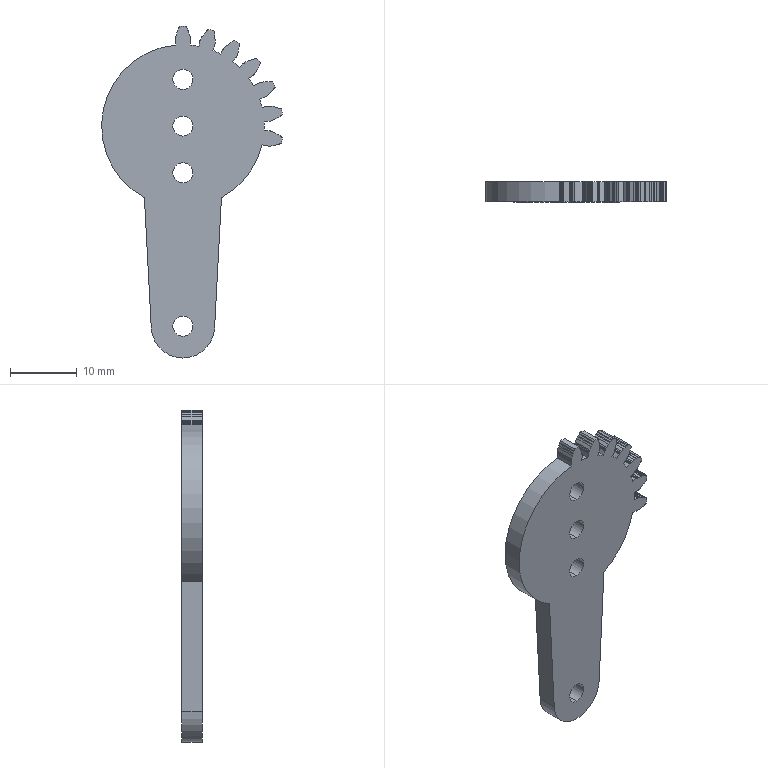Part | STEP file | Claw gear 2 | 1 solid | 253 faces | box 27.091 x 3 x 49.757 mm | volume 2108 mm3 | plane 186 | cylinder 67 | commonest cylinder face diameters 5.449 x14 17.652 x14 33.818 x14 3 x8 24.375 x8 30 x7